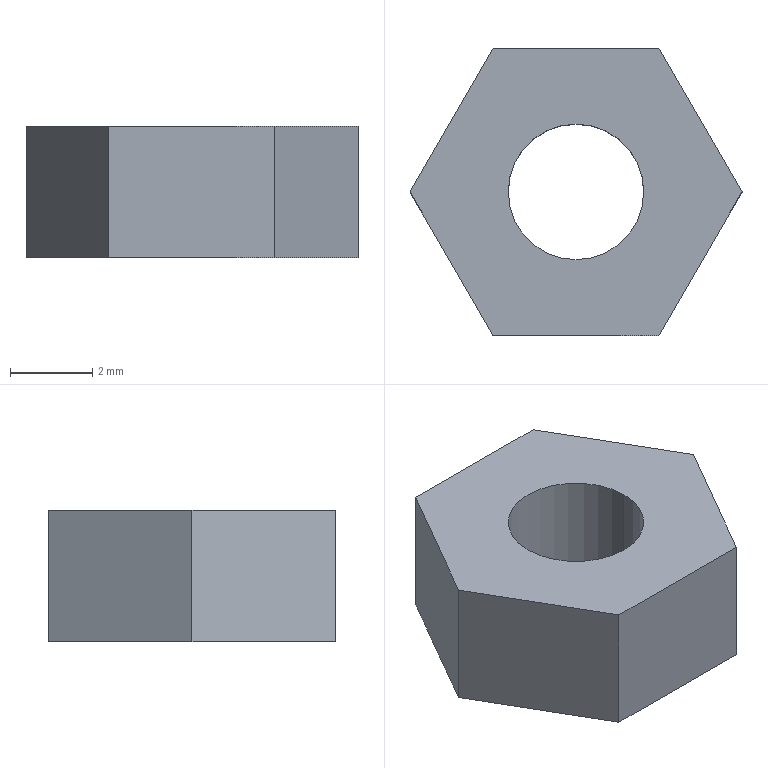Part | SolidWorks | features Extrusion 1 | 1 solid | 10 faces | box 8.083 x 7 x 3.2 mm | volume 108.423 mm3 | plane 8 | cylinder 2 | commonest cylinder face diameters 3.3 x2
STEP:
#1=CARTESIAN_POINT('',(-1.65,0.,-1.6));
#2=VERTEX_POINT('',#1);
#3=CARTESIAN_POINT('',(1.65,0.,-1.6));
#4=VERTEX_POINT('',#3);
#5=CARTESIAN_POINT('',(0.,0.,-1.6));
#6=DIRECTION('',(0.,0.,1.));
#7=DIRECTION('',(1.,0.,0.));
#8=AXIS2_PLACEMENT_3D('',#5,#6,#7);
#9=CIRCLE('',#8,1.65);
#10=EDGE_CURVE('',#2,#4,#9,.T.);
#11=ORIENTED_EDGE('',*,*,#10,.F.);
#12=CARTESIAN_POINT('',(-1.65,0.,1.6));
#13=VERTEX_POINT('',#12);
#14=CARTESIAN_POINT('',(-1.65,0.,-1.6));
#15=DIRECTION('',(0.,0.,1.));
#16=VECTOR('',#15,1000.);
#17=LINE('',#14,#16);
#18=EDGE_CURVE('',#2,#13,#17,.T.);
#19=ORIENTED_EDGE('',*,*,#18,.T.);
#20=CARTESIAN_POINT('',(1.65,0.,1.6));
#21=VERTEX_POINT('',#20);
#22=CARTESIAN_POINT('',(0.,0.,1.6));
#23=DIRECTION('',(0.,0.,1.));
#24=DIRECTION('',(1.,0.,0.));
#25=AXIS2_PLACEMENT_3D('',#22,#23,#24);
#26=CIRCLE('',#25,1.65);
#27=EDGE_CURVE('',#13,#21,#26,.T.);
#28=ORIENTED_EDGE('',*,*,#27,.T.);
#29=CARTESIAN_POINT('',(1.65,0.,-1.6));
#30=DIRECTION('',(0.,0.,1.));
#31=VECTOR('',#30,1000.);
#32=LINE('',#29,#31);
#33=EDGE_CURVE('',#4,#21,#32,.T.);
#34=ORIENTED_EDGE('',*,*,#33,.F.);
#35=EDGE_LOOP('',(#11,#19,#28,#34));
#36=FACE_OUTER_BOUND('',#35,.T.);
#37=CARTESIAN_POINT('',(0.,0.,-1.6));
#38=DIRECTION('',(0.,0.,1.));
#39=DIRECTION('',(1.,0.,0.));
#40=AXIS2_PLACEMENT_3D('',#37,#38,#39);
#41=CYLINDRICAL_SURFACE('',#40,1.65);
#42=ADVANCED_FACE('',(#36),#41,.F.);
#43=CARTESIAN_POINT('',(2.021,-3.5,1.6));
#44=VERTEX_POINT('',#43);
#45=CARTESIAN_POINT('',(4.041,0.,1.6));
#46=VERTEX_POINT('',#45);
#47=CARTESIAN_POINT('',(2.021,-3.5,1.6));
#48=DIRECTION('',(0.5,0.866,0.));
#49=VECTOR('',#48,1000.);
#50=LINE('',#47,#49);
#51=EDGE_CURVE('',#44,#46,#50,.T.);
#52=ORIENTED_EDGE('',*,*,#51,.F.);
#53=CARTESIAN_POINT('',(2.021,-3.5,-1.6));
#54=VERTEX_POINT('',#53);
#55=CARTESIAN_POINT('',(2.021,-3.5,-1.6));
#56=DIRECTION('',(0.,0.,1.));
#57=VECTOR('',#56,1000.);
#58=LINE('',#55,#57);
#59=EDGE_CURVE('',#54,#44,#58,.T.);
#60=ORIENTED_EDGE('',*,*,#59,.F.);
#61=CARTESIAN_POINT('',(4.041,0.,-1.6));
#62=VERTEX_POINT('',#61);
#63=CARTESIAN_POINT('',(2.021,-3.5,-1.6));
#64=DIRECTION('',(0.5,0.866,0.));
#65=VECTOR('',#64,1000.);
#66=LINE('',#63,#65);
#67=EDGE_CURVE('',#54,#62,#66,.T.);
#68=ORIENTED_EDGE('',*,*,#67,.T.);
#69=CARTESIAN_POINT('',(4.041,0.,-1.6));
#70=DIRECTION('',(0.,0.,1.));
#71=VECTOR('',#70,1000.);
#72=LINE('',#69,#71);
#73=EDGE_CURVE('',#62,#46,#72,.T.);
#74=ORIENTED_EDGE('',*,*,#73,.T.);
#75=EDGE_LOOP('',(#52,#60,#68,#74));
#76=FACE_OUTER_BOUND('',#75,.T.);
#77=CARTESIAN_POINT('',(2.021,-3.5,-1.6));
#78=DIRECTION('',(0.866,-0.5,0.));
#79=DIRECTION('',(0.5,0.866,0.));
#80=AXIS2_PLACEMENT_3D('',#77,#78,#79);
#81=PLANE('',#80);
#82=ADVANCED_FACE('',(#76),#81,.T.);
#83=CARTESIAN_POINT('',(-2.021,-3.5,1.6));
#84=VERTEX_POINT('',#83);
#85=CARTESIAN_POINT('',(-2.021,-3.5,1.6));
#86=DIRECTION('',(1.,0.,0.));
#87=VECTOR('',#86,1000.);
#88=LINE('',#85,#87);
#89=EDGE_CURVE('',#84,#44,#88,.T.);
#90=ORIENTED_EDGE('',*,*,#89,.F.);
#91=CARTESIAN_POINT('',(-2.021,-3.5,-1.6));
#92=VERTEX_POINT('',#91);
#93=CARTESIAN_POINT('',(-2.021,-3.5,-1.6));
#94=DIRECTION('',(0.,0.,1.));
#95=VECTOR('',#94,1000.);
#96=LINE('',#93,#95);
#97=EDGE_CURVE('',#92,#84,#96,.T.);
#98=ORIENTED_EDGE('',*,*,#97,.F.);
#99=CARTESIAN_POINT('',(-2.021,-3.5,-1.6));
#100=DIRECTION('',(1.,0.,0.));
#101=VECTOR('',#100,1000.);
#102=LINE('',#99,#101);
#103=EDGE_CURVE('',#92,#54,#102,.T.);
#104=ORIENTED_EDGE('',*,*,#103,.T.);
#105=ORIENTED_EDGE('',*,*,#59,.T.);
#106=EDGE_LOOP('',(#90,#98,#104,#105));
#107=FACE_OUTER_BOUND('',#106,.T.);
#108=CARTESIAN_POINT('',(-2.021,-3.5,-1.6));
#109=DIRECTION('',(0.,-1.,0.));
#110=DIRECTION('',(1.,0.,0.));
#111=AXIS2_PLACEMENT_3D('',#108,#109,#110);
#112=PLANE('',#111);
#113=ADVANCED_FACE('',(#107),#112,.T.);
#114=CARTESIAN_POINT('',(-4.041,0.,1.6));
#115=VERTEX_POINT('',#114);
#116=CARTESIAN_POINT('',(-4.041,0.,1.6));
#117=DIRECTION('',(0.5,-0.866,0.));
#118=VECTOR('',#117,1000.);
#119=LINE('',#116,#118);
#120=EDGE_CURVE('',#115,#84,#119,.T.);
#121=ORIENTED_EDGE('',*,*,#120,.F.);
#122=CARTESIAN_POINT('',(-4.041,0.,-1.6));
#123=VERTEX_POINT('',#122);
#124=CARTESIAN_POINT('',(-4.041,0.,-1.6));
#125=DIRECTION('',(0.,0.,1.));
#126=VECTOR('',#125,1000.);
#127=LINE('',#124,#126);
#128=EDGE_CURVE('',#123,#115,#127,.T.);
#129=ORIENTED_EDGE('',*,*,#128,.F.);
#130=CARTESIAN_POINT('',(-4.041,0.,-1.6));
#131=DIRECTION('',(0.5,-0.866,0.));
#132=VECTOR('',#131,1000.);
#133=LINE('',#130,#132);
#134=EDGE_CURVE('',#123,#92,#133,.T.);
#135=ORIENTED_EDGE('',*,*,#134,.T.);
#136=ORIENTED_EDGE('',*,*,#97,.T.);
#137=EDGE_LOOP('',(#121,#129,#135,#136));
#138=FACE_OUTER_BOUND('',#137,.T.);
#139=CARTESIAN_POINT('',(-4.041,0.,-1.6));
#140=DIRECTION('',(-0.866,-0.5,0.));
#141=DIRECTION('',(0.5,-0.866,0.));
#142=AXIS2_PLACEMENT_3D('',#139,#140,#141);
#143=PLANE('',#142);
#144=ADVANCED_FACE('',(#138),#143,.T.);
#145=CARTESIAN_POINT('',(-2.021,3.5,1.6));
#146=VERTEX_POINT('',#145);
#147=CARTESIAN_POINT('',(-2.021,3.5,1.6));
#148=DIRECTION('',(-0.5,-0.866,0.));
#149=VECTOR('',#148,1000.);
#150=LINE('',#147,#149);
#151=EDGE_CURVE('',#146,#115,#150,.T.);
#152=ORIENTED_EDGE('',*,*,#151,.F.);
#153=CARTESIAN_POINT('',(-2.021,3.5,-1.6));
#154=VERTEX_POINT('',#153);
#155=CARTESIAN_POINT('',(-2.021,3.5,-1.6));
#156=DIRECTION('',(0.,0.,1.));
#157=VECTOR('',#156,1000.);
#158=LINE('',#155,#157);
#159=EDGE_CURVE('',#154,#146,#158,.T.);
#160=ORIENTED_EDGE('',*,*,#159,.F.);
#161=CARTESIAN_POINT('',(-2.021,3.5,-1.6));
#162=DIRECTION('',(-0.5,-0.866,0.));
#163=VECTOR('',#162,1000.);
#164=LINE('',#161,#163);
#165=EDGE_CURVE('',#154,#123,#164,.T.);
#166=ORIENTED_EDGE('',*,*,#165,.T.);
#167=ORIENTED_EDGE('',*,*,#128,.T.);
#168=EDGE_LOOP('',(#152,#160,#166,#167));
#169=FACE_OUTER_BOUND('',#168,.T.);
#170=CARTESIAN_POINT('',(-2.021,3.5,-1.6));
#171=DIRECTION('',(-0.866,0.5,0.));
#172=DIRECTION('',(-0.5,-0.866,0.));
#173=AXIS2_PLACEMENT_3D('',#170,#171,#172);
#174=PLANE('',#173);
#175=ADVANCED_FACE('',(#169),#174,.T.);
#176=CARTESIAN_POINT('',(2.021,3.5,1.6));
#177=VERTEX_POINT('',#176);
#178=CARTESIAN_POINT('',(2.021,3.5,1.6));
#179=DIRECTION('',(-1.,0.,0.));
#180=VECTOR('',#179,1000.);
#181=LINE('',#178,#180);
#182=EDGE_CURVE('',#177,#146,#181,.T.);
#183=ORIENTED_EDGE('',*,*,#182,.F.);
#184=CARTESIAN_POINT('',(2.021,3.5,-1.6));
#185=VERTEX_POINT('',#184);
#186=CARTESIAN_POINT('',(2.021,3.5,-1.6));
#187=DIRECTION('',(0.,0.,1.));
#188=VECTOR('',#187,1000.);
#189=LINE('',#186,#188);
#190=EDGE_CURVE('',#185,#177,#189,.T.);
#191=ORIENTED_EDGE('',*,*,#190,.F.);
#192=CARTESIAN_POINT('',(2.021,3.5,-1.6));
#193=DIRECTION('',(-1.,0.,0.));
#194=VECTOR('',#193,1000.);
#195=LINE('',#192,#194);
#196=EDGE_CURVE('',#185,#154,#195,.T.);
#197=ORIENTED_EDGE('',*,*,#196,.T.);
#198=ORIENTED_EDGE('',*,*,#159,.T.);
#199=EDGE_LOOP('',(#183,#191,#197,#198));
#200=FACE_OUTER_BOUND('',#199,.T.);
#201=CARTESIAN_POINT('',(2.021,3.5,-1.6));
#202=DIRECTION('',(0.,1.,0.));
#203=DIRECTION('',(-1.,0.,0.));
#204=AXIS2_PLACEMENT_3D('',#201,#202,#203);
#205=PLANE('',#204);
#206=ADVANCED_FACE('',(#200),#205,.T.);
#207=CARTESIAN_POINT('',(4.041,0.,1.6));
#208=DIRECTION('',(-0.5,0.866,0.));
#209=VECTOR('',#208,1000.);
#210=LINE('',#207,#209);
#211=EDGE_CURVE('',#46,#177,#210,.T.);
#212=ORIENTED_EDGE('',*,*,#211,.F.);
#213=ORIENTED_EDGE('',*,*,#73,.F.);
#214=CARTESIAN_POINT('',(4.041,0.,-1.6));
#215=DIRECTION('',(-0.5,0.866,0.));
#216=VECTOR('',#215,1000.);
#217=LINE('',#214,#216);
#218=EDGE_CURVE('',#62,#185,#217,.T.);
#219=ORIENTED_EDGE('',*,*,#218,.T.);
#220=ORIENTED_EDGE('',*,*,#190,.T.);
#221=EDGE_LOOP('',(#212,#213,#219,#220));
#222=FACE_OUTER_BOUND('',#221,.T.);
#223=CARTESIAN_POINT('',(4.041,0.,-1.6));
#224=DIRECTION('',(0.866,0.5,0.));
#225=DIRECTION('',(-0.5,0.866,0.));
#226=AXIS2_PLACEMENT_3D('',#223,#224,#225);
#227=PLANE('',#226);
#228=ADVANCED_FACE('',(#222),#227,.T.);
#229=CARTESIAN_POINT('',(0.,0.,-1.6));
#230=DIRECTION('',(0.,0.,1.));
#231=DIRECTION('',(1.,0.,0.));
#232=AXIS2_PLACEMENT_3D('',#229,#230,#231);
#233=CIRCLE('',#232,1.65);
#234=EDGE_CURVE('',#4,#2,#233,.T.);
#235=ORIENTED_EDGE('',*,*,#234,.T.);
#236=ORIENTED_EDGE('',*,*,#10,.T.);
#237=EDGE_LOOP('',(#235,#236));
#238=FACE_BOUND('',#237,.T.);
#239=ORIENTED_EDGE('',*,*,#67,.F.);
#240=ORIENTED_EDGE('',*,*,#103,.F.);
#241=ORIENTED_EDGE('',*,*,#134,.F.);
#242=ORIENTED_EDGE('',*,*,#165,.F.);
#243=ORIENTED_EDGE('',*,*,#196,.F.);
#244=ORIENTED_EDGE('',*,*,#218,.F.);
#245=EDGE_LOOP('',(#239,#240,#241,#242,#243,#244));
#246=FACE_OUTER_BOUND('',#245,.T.);
#247=CARTESIAN_POINT('',(0.,0.,-1.6));
#248=DIRECTION('',(0.,0.,1.));
#249=DIRECTION('',(1.,0.,0.));
#250=AXIS2_PLACEMENT_3D('',#247,#248,#249);
#251=PLANE('',#250);
#252=ADVANCED_FACE('',(#238,#246),#251,.F.);
#253=CARTESIAN_POINT('',(0.,0.,1.6));
#254=DIRECTION('',(0.,0.,1.));
#255=DIRECTION('',(1.,0.,0.));
#256=AXIS2_PLACEMENT_3D('',#253,#254,#255);
#257=CIRCLE('',#256,1.65);
#258=EDGE_CURVE('',#21,#13,#257,.T.);
#259=ORIENTED_EDGE('',*,*,#258,.F.);
#260=ORIENTED_EDGE('',*,*,#27,.F.);
#261=EDGE_LOOP('',(#259,#260));
#262=FACE_BOUND('',#261,.T.);
#263=ORIENTED_EDGE('',*,*,#51,.T.);
#264=ORIENTED_EDGE('',*,*,#211,.T.);
#265=ORIENTED_EDGE('',*,*,#182,.T.);
#266=ORIENTED_EDGE('',*,*,#151,.T.);
#267=ORIENTED_EDGE('',*,*,#120,.T.);
#268=ORIENTED_EDGE('',*,*,#89,.T.);
#269=EDGE_LOOP('',(#263,#264,#265,#266,#267,#268));
#270=FACE_OUTER_BOUND('',#269,.T.);
#271=CARTESIAN_POINT('',(0.,0.,1.6));
#272=DIRECTION('',(0.,0.,1.));
#273=DIRECTION('',(1.,0.,0.));
#274=AXIS2_PLACEMENT_3D('',#271,#272,#273);
#275=PLANE('',#274);
#276=ADVANCED_FACE('',(#262,#270),#275,.T.);
#277=ORIENTED_EDGE('',*,*,#18,.F.);
#278=ORIENTED_EDGE('',*,*,#234,.F.);
#279=ORIENTED_EDGE('',*,*,#33,.T.);
#280=ORIENTED_EDGE('',*,*,#258,.T.);
#281=EDGE_LOOP('',(#277,#278,#279,#280));
#282=FACE_OUTER_BOUND('',#281,.T.);
#283=CARTESIAN_POINT('',(0.,0.,-1.6));
#284=DIRECTION('',(0.,0.,1.));
#285=DIRECTION('',(1.,0.,0.));
#286=AXIS2_PLACEMENT_3D('',#283,#284,#285);
#287=CYLINDRICAL_SURFACE('',#286,1.65);
#288=ADVANCED_FACE('',(#282),#287,.F.);
#289=CLOSED_SHELL('',(#42,#82,#113,#144,#175,#206,#228,#252,#276,#288));
#290=MANIFOLD_SOLID_BREP('',#289);
#291=CARTESIAN_POINT('',(0.,0.,0.));
#292=DIRECTION('',(0.,0.,1.));
#293=DIRECTION('',(1.,0.,0.));
#294=AXIS2_PLACEMENT_3D('',#291,#292,#293);
#295=(LENGTH_UNIT()NAMED_UNIT(*)SI_UNIT(.MILLI.,.METRE.));
#296=UNCERTAINTY_MEASURE_WITH_UNIT(LENGTH_MEASURE(0.00001),#295,'','');
#297=(NAMED_UNIT(*)PLANE_ANGLE_UNIT()SI_UNIT($,.RADIAN.));
#298=(NAMED_UNIT(*)SI_UNIT($,.STERADIAN.)SOLID_ANGLE_UNIT());
#299=(GEOMETRIC_REPRESENTATION_CONTEXT(3)GLOBAL_UNCERTAINTY_ASSIGNED_CONTEXT((#296))GLOBAL_UNIT_ASSIGNED_CONTEXT((#295,#297,#298))REPRESENTATION_CONTEXT('',''));
#300=ADVANCED_BREP_SHAPE_REPRESENTATION('',(#290,#294),#299);